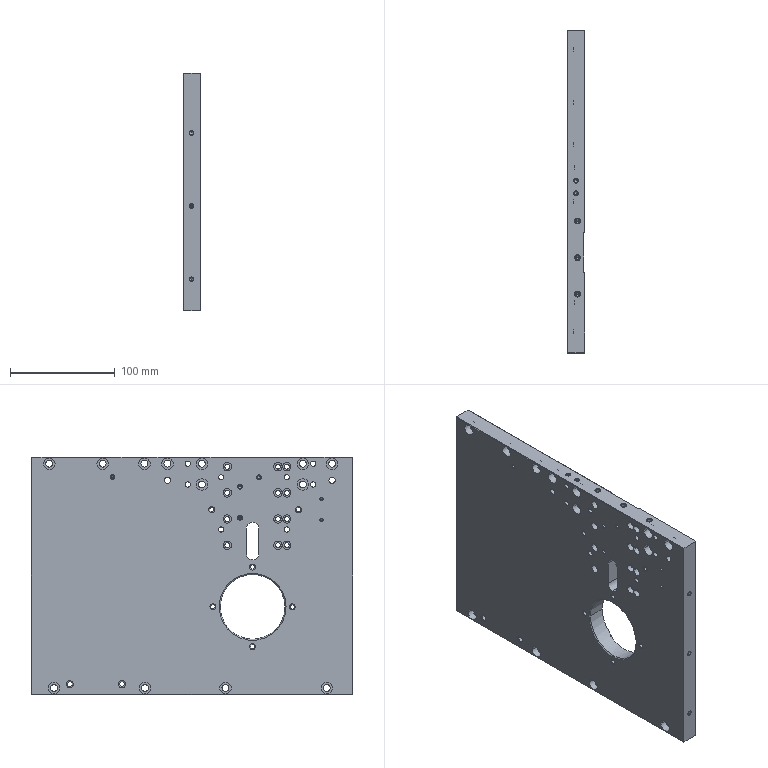Part | NX | 1 solid | 310 faces | box 17 x 308 x 227 mm | volume 1095809 mm3 | cylinder 175 | cone 86 | plane 49 | commonest cylinder face diameters 6.6 x26 11 x26 8 x24 5 x20 3.3 x18 4.2 x18